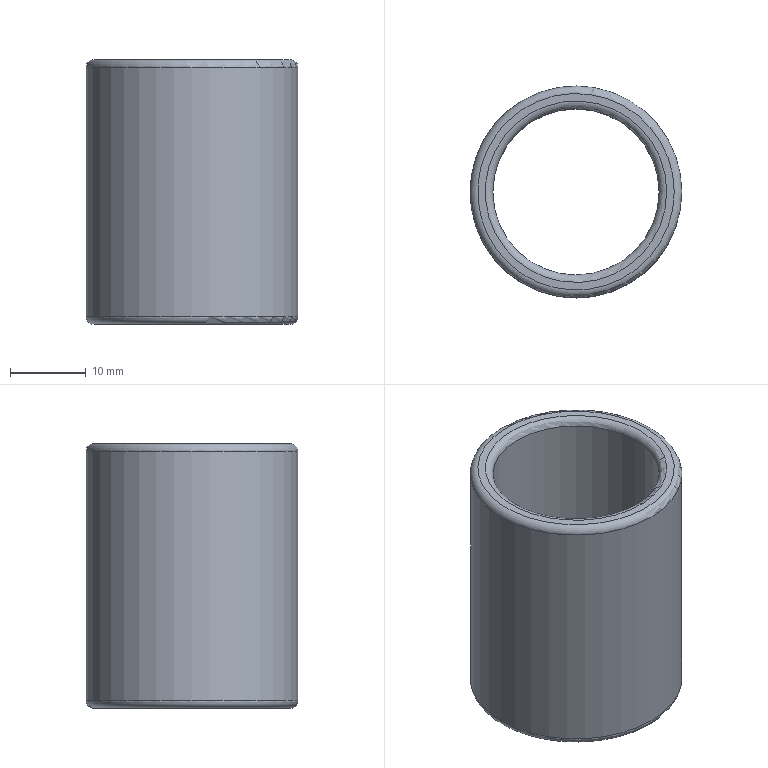Part | STEP file | 1 solid | 8 faces | box 28 x 28 x 35 mm | volume 8179 mm3 | torus 4 | plane 2 | cylinder 2 | commonest cylinder face diameters 22 x1 28 x1
STEP:
#1=CARTESIAN_POINT('',(0.,0.,0.));
#2=DIRECTION('',(0.,0.,1.));
#3=DIRECTION('',(1.,0.,0.));
#4=AXIS2_PLACEMENT_3D('',#1,#2,#3);
#5=CARTESIAN_POINT('',(1547.247,368.48,38.619));
#6=VERTEX_POINT('',#5);
#7=CARTESIAN_POINT('',(1534.247,368.48,38.619));
#8=DIRECTION('',(0.,0.,1.));
#9=DIRECTION('',(1.,0.,0.));
#10=AXIS2_PLACEMENT_3D('',#7,#8,#9);
#11=CIRCLE('',#10,13.);
#12=CARTESIAN_POINT('',(1534.247,368.48,38.619));
#13=DIRECTION('',(0.,0.,1.));
#14=DIRECTION('',(1.,0.,0.));
#15=AXIS2_PLACEMENT_3D('',#12,#13,#14);
#16=PLANE('',#15);
#17=CARTESIAN_POINT('',(0.,0.));
#18=DIRECTION('',(1.,0.));
#19=AXIS2_PLACEMENT_2D('',#17,#18);
#20=CIRCLE('',#19,13.);
#21=(GEOMETRIC_REPRESENTATION_CONTEXT(2)PARAMETRIC_REPRESENTATION_CONTEXT()REPRESENTATION_CONTEXT('',''));
#22=DEFINITIONAL_REPRESENTATION('',(#20),#21);
#23=PCURVE('',#16,#22);
#24=CARTESIAN_POINT('',(1534.247,368.48,37.619));
#25=DIRECTION('',(0.,0.,1.));
#26=DIRECTION('',(-1.,0.,0.));
#27=AXIS2_PLACEMENT_3D('',#24,#25,#26);
#28=TOROIDAL_SURFACE('',#27,13.,1.);
#29=CARTESIAN_POINT('',(3.142,7.854));
#30=DIRECTION('',(1.,0.));
#31=VECTOR('',#30,1.);
#32=LINE('',#29,#31);
#33=(GEOMETRIC_REPRESENTATION_CONTEXT(2)PARAMETRIC_REPRESENTATION_CONTEXT()REPRESENTATION_CONTEXT('',''));
#34=DEFINITIONAL_REPRESENTATION('',(#32),#33);
#35=PCURVE('',#28,#34);
#36=SURFACE_CURVE('',#11,(#23,#35),.PCURVE_S1.);
#37=EDGE_CURVE('',#6,#6,#36,.T.);
#38=ORIENTED_EDGE('',*,*,#37,.T.);
#39=EDGE_LOOP('',(#38));
#40=FACE_BOUND('',#39,.T.);
#41=CARTESIAN_POINT('',(1546.247,368.48,38.619));
#42=VERTEX_POINT('',#41);
#43=CARTESIAN_POINT('',(1534.247,368.48,38.619));
#44=DIRECTION('',(0.,0.,-1.));
#45=DIRECTION('',(1.,0.,0.));
#46=AXIS2_PLACEMENT_3D('',#43,#44,#45);
#47=CIRCLE('',#46,12.);
#48=CARTESIAN_POINT('',(12.,0.));
#49=CARTESIAN_POINT('',(12.,-20.785));
#50=CARTESIAN_POINT('',(-6.,-10.392));
#51=CARTESIAN_POINT('',(-24.,0.));
#52=CARTESIAN_POINT('',(-6.,10.392));
#53=CARTESIAN_POINT('',(12.,20.785));
#54=CARTESIAN_POINT('',(12.,0.));
#55=(BOUNDED_CURVE()B_SPLINE_CURVE(2,(#48,#49,#50,#51,#52,#53,#54),.UNSPECIFIED.,.T.,.F.)B_SPLINE_CURVE_WITH_KNOTS((1,2,2,2,2,1),(-2.094,0.,2.094,4.189,6.283,8.378),.UNSPECIFIED.)CURVE()GEOMETRIC_REPRESENTATION_ITEM()RATIONAL_B_SPLINE_CURVE((1.,0.5,1.,0.5,1.,0.5,1.))REPRESENTATION_ITEM(''));
#56=(GEOMETRIC_REPRESENTATION_CONTEXT(2)PARAMETRIC_REPRESENTATION_CONTEXT()REPRESENTATION_CONTEXT('',''));
#57=DEFINITIONAL_REPRESENTATION('',(#55),#56);
#58=PCURVE('',#16,#57);
#59=CARTESIAN_POINT('',(1534.247,368.48,37.619));
#60=DIRECTION('',(0.,0.,1.));
#61=DIRECTION('',(-1.,0.,0.));
#62=AXIS2_PLACEMENT_3D('',#59,#60,#61);
#63=TOROIDAL_SURFACE('',#62,12.,1.);
#64=CARTESIAN_POINT('',(9.425,7.854));
#65=DIRECTION('',(-1.,0.));
#66=VECTOR('',#65,1.);
#67=LINE('',#64,#66);
#68=(GEOMETRIC_REPRESENTATION_CONTEXT(2)PARAMETRIC_REPRESENTATION_CONTEXT()REPRESENTATION_CONTEXT('',''));
#69=DEFINITIONAL_REPRESENTATION('',(#67),#68);
#70=PCURVE('',#63,#69);
#71=SURFACE_CURVE('',#47,(#58,#70),.PCURVE_S1.);
#72=EDGE_CURVE('',#42,#42,#71,.T.);
#73=ORIENTED_EDGE('',*,*,#72,.T.);
#74=EDGE_LOOP('',(#73));
#75=FACE_BOUND('',#74,.T.);
#76=ADVANCED_FACE('',(#40,#75),#16,.T.);
#77=CARTESIAN_POINT('',(1548.247,368.48,37.619));
#78=VERTEX_POINT('',#77);
#79=CARTESIAN_POINT('',(1534.247,368.48,37.619));
#80=DIRECTION('',(0.,0.,-1.));
#81=DIRECTION('',(1.,0.,0.));
#82=AXIS2_PLACEMENT_3D('',#79,#80,#81);
#83=CIRCLE('',#82,14.);
#84=CARTESIAN_POINT('',(1534.247,368.48,33.619));
#85=DIRECTION('',(0.,0.,-1.));
#86=DIRECTION('',(-1.,0.,0.));
#87=AXIS2_PLACEMENT_3D('',#84,#85,#86);
#88=CYLINDRICAL_SURFACE('',#87,14.);
#89=CARTESIAN_POINT('',(3.142,-4.));
#90=DIRECTION('',(1.,0.));
#91=VECTOR('',#90,1.);
#92=LINE('',#89,#91);
#93=(GEOMETRIC_REPRESENTATION_CONTEXT(2)PARAMETRIC_REPRESENTATION_CONTEXT()REPRESENTATION_CONTEXT('',''));
#94=DEFINITIONAL_REPRESENTATION('',(#92),#93);
#95=PCURVE('',#88,#94);
#96=CARTESIAN_POINT('',(9.425,6.283));
#97=DIRECTION('',(-1.,0.));
#98=VECTOR('',#97,1.);
#99=LINE('',#96,#98);
#100=(GEOMETRIC_REPRESENTATION_CONTEXT(2)PARAMETRIC_REPRESENTATION_CONTEXT()REPRESENTATION_CONTEXT('',''));
#101=DEFINITIONAL_REPRESENTATION('',(#99),#100);
#102=PCURVE('',#28,#101);
#103=SURFACE_CURVE('',#83,(#95,#102),.PCURVE_S1.);
#104=EDGE_CURVE('',#78,#78,#103,.T.);
#105=ORIENTED_EDGE('',*,*,#104,.T.);
#106=CARTESIAN_POINT('',(1548.247,368.48,4.619));
#107=VERTEX_POINT('',#106);
#108=CARTESIAN_POINT('',(1548.247,368.48,37.619));
#109=CARTESIAN_POINT('',(1548.247,368.48,4.619));
#110=B_SPLINE_CURVE_WITH_KNOTS('',1,(#108,#109),.UNSPECIFIED.,.F.,.F.,(2,2),(-4.,29.),.PIECEWISE_BEZIER_KNOTS.);
#111=CARTESIAN_POINT('',(9.425,0.));
#112=DIRECTION('',(0.,1.));
#113=VECTOR('',#112,1.);
#114=LINE('',#111,#113);
#115=(GEOMETRIC_REPRESENTATION_CONTEXT(2)PARAMETRIC_REPRESENTATION_CONTEXT()REPRESENTATION_CONTEXT('',''));
#116=DEFINITIONAL_REPRESENTATION('',(#114),#115);
#117=PCURVE('',#88,#116);
#118=CARTESIAN_POINT('',(3.142,0.));
#119=DIRECTION('',(0.,1.));
#120=VECTOR('',#119,1.);
#121=LINE('',#118,#120);
#122=(GEOMETRIC_REPRESENTATION_CONTEXT(2)PARAMETRIC_REPRESENTATION_CONTEXT()REPRESENTATION_CONTEXT('',''));
#123=DEFINITIONAL_REPRESENTATION('',(#121),#122);
#124=PCURVE('',#88,#123);
#125=SEAM_CURVE('',#110,(#117,#124),.PCURVE_S1.);
#126=EDGE_CURVE('',#78,#107,#125,.T.);
#127=ORIENTED_EDGE('',*,*,#126,.T.);
#128=CARTESIAN_POINT('',(1534.247,368.48,4.619));
#129=DIRECTION('',(0.,0.,1.));
#130=DIRECTION('',(1.,0.,0.));
#131=AXIS2_PLACEMENT_3D('',#128,#129,#130);
#132=CIRCLE('',#131,14.);
#133=CARTESIAN_POINT('',(9.425,29.));
#134=DIRECTION('',(-1.,0.));
#135=VECTOR('',#134,1.);
#136=LINE('',#133,#135);
#137=(GEOMETRIC_REPRESENTATION_CONTEXT(2)PARAMETRIC_REPRESENTATION_CONTEXT()REPRESENTATION_CONTEXT('',''));
#138=DEFINITIONAL_REPRESENTATION('',(#136),#137);
#139=PCURVE('',#88,#138);
#140=CARTESIAN_POINT('',(1534.247,368.48,4.619));
#141=DIRECTION('',(0.,0.,1.));
#142=DIRECTION('',(-1.,0.,0.));
#143=AXIS2_PLACEMENT_3D('',#140,#141,#142);
#144=TOROIDAL_SURFACE('',#143,13.,1.);
#145=CARTESIAN_POINT('',(3.142,6.283));
#146=DIRECTION('',(1.,0.));
#147=VECTOR('',#146,1.);
#148=LINE('',#145,#147);
#149=(GEOMETRIC_REPRESENTATION_CONTEXT(2)PARAMETRIC_REPRESENTATION_CONTEXT()REPRESENTATION_CONTEXT('',''));
#150=DEFINITIONAL_REPRESENTATION('',(#148),#149);
#151=PCURVE('',#144,#150);
#152=SURFACE_CURVE('',#132,(#139,#151),.PCURVE_S1.);
#153=EDGE_CURVE('',#107,#107,#152,.T.);
#154=ORIENTED_EDGE('',*,*,#153,.T.);
#155=ORIENTED_EDGE('',*,*,#126,.F.);
#156=EDGE_LOOP('',(#105,#127,#154,#155));
#157=FACE_BOUND('',#156,.T.);
#158=ADVANCED_FACE('',(#157),#88,.T.);
#159=CARTESIAN_POINT('',(1546.247,368.48,3.619));
#160=VERTEX_POINT('',#159);
#161=CARTESIAN_POINT('',(1534.247,368.48,3.619));
#162=DIRECTION('',(0.,0.,1.));
#163=DIRECTION('',(1.,0.,0.));
#164=AXIS2_PLACEMENT_3D('',#161,#162,#163);
#165=CIRCLE('',#164,12.);
#166=CARTESIAN_POINT('',(1534.247,368.48,3.619));
#167=DIRECTION('',(0.,0.,1.));
#168=DIRECTION('',(1.,0.,0.));
#169=AXIS2_PLACEMENT_3D('',#166,#167,#168);
#170=PLANE('',#169);
#171=CARTESIAN_POINT('',(0.,0.));
#172=DIRECTION('',(1.,0.));
#173=AXIS2_PLACEMENT_2D('',#171,#172);
#174=CIRCLE('',#173,12.);
#175=(GEOMETRIC_REPRESENTATION_CONTEXT(2)PARAMETRIC_REPRESENTATION_CONTEXT()REPRESENTATION_CONTEXT('',''));
#176=DEFINITIONAL_REPRESENTATION('',(#174),#175);
#177=PCURVE('',#170,#176);
#178=CARTESIAN_POINT('',(1534.247,368.48,4.619));
#179=DIRECTION('',(0.,0.,1.));
#180=DIRECTION('',(-1.,0.,0.));
#181=AXIS2_PLACEMENT_3D('',#178,#179,#180);
#182=TOROIDAL_SURFACE('',#181,12.,1.);
#183=CARTESIAN_POINT('',(3.142,4.712));
#184=DIRECTION('',(1.,0.));
#185=VECTOR('',#184,1.);
#186=LINE('',#183,#185);
#187=(GEOMETRIC_REPRESENTATION_CONTEXT(2)PARAMETRIC_REPRESENTATION_CONTEXT()REPRESENTATION_CONTEXT('',''));
#188=DEFINITIONAL_REPRESENTATION('',(#186),#187);
#189=PCURVE('',#182,#188);
#190=SURFACE_CURVE('',#165,(#177,#189),.PCURVE_S1.);
#191=EDGE_CURVE('',#160,#160,#190,.T.);
#192=ORIENTED_EDGE('',*,*,#191,.T.);
#193=EDGE_LOOP('',(#192));
#194=FACE_BOUND('',#193,.T.);
#195=CARTESIAN_POINT('',(1547.247,368.48,3.619));
#196=VERTEX_POINT('',#195);
#197=CARTESIAN_POINT('',(1534.247,368.48,3.619));
#198=DIRECTION('',(0.,0.,-1.));
#199=DIRECTION('',(1.,0.,0.));
#200=AXIS2_PLACEMENT_3D('',#197,#198,#199);
#201=CIRCLE('',#200,13.);
#202=CARTESIAN_POINT('',(13.,0.));
#203=CARTESIAN_POINT('',(13.,-22.517));
#204=CARTESIAN_POINT('',(-6.5,-11.258));
#205=CARTESIAN_POINT('',(-26.,0.));
#206=CARTESIAN_POINT('',(-6.5,11.258));
#207=CARTESIAN_POINT('',(13.,22.517));
#208=CARTESIAN_POINT('',(13.,0.));
#209=(BOUNDED_CURVE()B_SPLINE_CURVE(2,(#202,#203,#204,#205,#206,#207,#208),.UNSPECIFIED.,.T.,.F.)B_SPLINE_CURVE_WITH_KNOTS((1,2,2,2,2,1),(-2.094,0.,2.094,4.189,6.283,8.378),.UNSPECIFIED.)CURVE()GEOMETRIC_REPRESENTATION_ITEM()RATIONAL_B_SPLINE_CURVE((1.,0.5,1.,0.5,1.,0.5,1.))REPRESENTATION_ITEM(''));
#210=(GEOMETRIC_REPRESENTATION_CONTEXT(2)PARAMETRIC_REPRESENTATION_CONTEXT()REPRESENTATION_CONTEXT('',''));
#211=DEFINITIONAL_REPRESENTATION('',(#209),#210);
#212=PCURVE('',#170,#211);
#213=CARTESIAN_POINT('',(9.425,4.712));
#214=DIRECTION('',(-1.,0.));
#215=VECTOR('',#214,1.);
#216=LINE('',#213,#215);
#217=(GEOMETRIC_REPRESENTATION_CONTEXT(2)PARAMETRIC_REPRESENTATION_CONTEXT()REPRESENTATION_CONTEXT('',''));
#218=DEFINITIONAL_REPRESENTATION('',(#216),#217);
#219=PCURVE('',#144,#218);
#220=SURFACE_CURVE('',#201,(#212,#219),.PCURVE_S1.);
#221=EDGE_CURVE('',#196,#196,#220,.T.);
#222=ORIENTED_EDGE('',*,*,#221,.T.);
#223=EDGE_LOOP('',(#222));
#224=FACE_BOUND('',#223,.T.);
#225=ADVANCED_FACE('',(#194,#224),#170,.F.);
#226=CARTESIAN_POINT('',(1545.247,368.48,37.619));
#227=VERTEX_POINT('',#226);
#228=CARTESIAN_POINT('',(1534.247,368.48,37.619));
#229=DIRECTION('',(0.,0.,1.));
#230=DIRECTION('',(1.,0.,0.));
#231=AXIS2_PLACEMENT_3D('',#228,#229,#230);
#232=CIRCLE('',#231,11.);
#233=CARTESIAN_POINT('',(1534.247,368.48,33.619));
#234=DIRECTION('',(0.,0.,-1.));
#235=DIRECTION('',(-1.,0.,0.));
#236=AXIS2_PLACEMENT_3D('',#233,#234,#235);
#237=CYLINDRICAL_SURFACE('',#236,11.);
#238=CARTESIAN_POINT('',(9.425,-4.));
#239=DIRECTION('',(-1.,0.));
#240=VECTOR('',#239,1.);
#241=LINE('',#238,#240);
#242=(GEOMETRIC_REPRESENTATION_CONTEXT(2)PARAMETRIC_REPRESENTATION_CONTEXT()REPRESENTATION_CONTEXT('',''));
#243=DEFINITIONAL_REPRESENTATION('',(#241),#242);
#244=PCURVE('',#237,#243);
#245=CARTESIAN_POINT('',(3.142,9.425));
#246=DIRECTION('',(1.,0.));
#247=VECTOR('',#246,1.);
#248=LINE('',#245,#247);
#249=(GEOMETRIC_REPRESENTATION_CONTEXT(2)PARAMETRIC_REPRESENTATION_CONTEXT()REPRESENTATION_CONTEXT('',''));
#250=DEFINITIONAL_REPRESENTATION('',(#248),#249);
#251=PCURVE('',#63,#250);
#252=SURFACE_CURVE('',#232,(#244,#251),.PCURVE_S1.);
#253=EDGE_CURVE('',#227,#227,#252,.T.);
#254=ORIENTED_EDGE('',*,*,#253,.F.);
#255=CARTESIAN_POINT('',(1545.247,368.48,4.619));
#256=VERTEX_POINT('',#255);
#257=CARTESIAN_POINT('',(1545.247,368.48,37.619));
#258=CARTESIAN_POINT('',(1545.247,368.48,4.619));
#259=B_SPLINE_CURVE_WITH_KNOTS('',1,(#257,#258),.UNSPECIFIED.,.F.,.F.,(2,2),(-4.,29.),.PIECEWISE_BEZIER_KNOTS.);
#260=CARTESIAN_POINT('',(9.425,0.));
#261=DIRECTION('',(0.,1.));
#262=VECTOR('',#261,1.);
#263=LINE('',#260,#262);
#264=(GEOMETRIC_REPRESENTATION_CONTEXT(2)PARAMETRIC_REPRESENTATION_CONTEXT()REPRESENTATION_CONTEXT('',''));
#265=DEFINITIONAL_REPRESENTATION('',(#263),#264);
#266=PCURVE('',#237,#265);
#267=CARTESIAN_POINT('',(3.142,0.));
#268=DIRECTION('',(0.,1.));
#269=VECTOR('',#268,1.);
#270=LINE('',#267,#269);
#271=(GEOMETRIC_REPRESENTATION_CONTEXT(2)PARAMETRIC_REPRESENTATION_CONTEXT()REPRESENTATION_CONTEXT('',''));
#272=DEFINITIONAL_REPRESENTATION('',(#270),#271);
#273=PCURVE('',#237,#272);
#274=SEAM_CURVE('',#259,(#266,#273),.PCURVE_S1.);
#275=EDGE_CURVE('',#227,#256,#274,.T.);
#276=ORIENTED_EDGE('',*,*,#275,.T.);
#277=CARTESIAN_POINT('',(1534.247,368.48,4.619));
#278=DIRECTION('',(0.,0.,-1.));
#279=DIRECTION('',(1.,0.,0.));
#280=AXIS2_PLACEMENT_3D('',#277,#278,#279);
#281=CIRCLE('',#280,11.);
#282=CARTESIAN_POINT('',(3.142,29.));
#283=DIRECTION('',(1.,0.));
#284=VECTOR('',#283,1.);
#285=LINE('',#282,#284);
#286=(GEOMETRIC_REPRESENTATION_CONTEXT(2)PARAMETRIC_REPRESENTATION_CONTEXT()REPRESENTATION_CONTEXT('',''));
#287=DEFINITIONAL_REPRESENTATION('',(#285),#286);
#288=PCURVE('',#237,#287);
#289=CARTESIAN_POINT('',(9.425,3.142));
#290=DIRECTION('',(-1.,0.));
#291=VECTOR('',#290,1.);
#292=LINE('',#289,#291);
#293=(GEOMETRIC_REPRESENTATION_CONTEXT(2)PARAMETRIC_REPRESENTATION_CONTEXT()REPRESENTATION_CONTEXT('',''));
#294=DEFINITIONAL_REPRESENTATION('',(#292),#293);
#295=PCURVE('',#182,#294);
#296=SURFACE_CURVE('',#281,(#288,#295),.PCURVE_S1.);
#297=EDGE_CURVE('',#256,#256,#296,.T.);
#298=ORIENTED_EDGE('',*,*,#297,.F.);
#299=ORIENTED_EDGE('',*,*,#275,.F.);
#300=EDGE_LOOP('',(#254,#276,#298,#299));
#301=FACE_BOUND('',#300,.F.);
#302=ADVANCED_FACE('',(#301),#237,.F.);
#303=ORIENTED_EDGE('',*,*,#104,.F.);
#304=CARTESIAN_POINT('',(1548.247,368.48,37.619));
#305=CARTESIAN_POINT('',(1548.247,368.48,37.886));
#306=CARTESIAN_POINT('',(1548.162,368.48,38.147));
#307=CARTESIAN_POINT('',(1547.999,368.48,38.371));
#308=CARTESIAN_POINT('',(1547.775,368.48,38.534));
#309=CARTESIAN_POINT('',(1547.515,368.48,38.619));
#310=CARTESIAN_POINT('',(1547.247,368.48,38.619));
#311=(BOUNDED_CURVE()B_SPLINE_CURVE(6,(#304,#305,#306,#307,#308,#309,#310),.UNSPECIFIED.,.F.,.F.)B_SPLINE_CURVE_WITH_KNOTS((7,7),(0.,1.571),.PIECEWISE_BEZIER_KNOTS.)CURVE()GEOMETRIC_REPRESENTATION_ITEM()RATIONAL_B_SPLINE_CURVE((1.031,1.01,0.9979,0.994,0.9979,1.01,1.031))REPRESENTATION_ITEM(''));
#312=CARTESIAN_POINT('',(9.425,6.283));
#313=DIRECTION('',(0.,1.));
#314=VECTOR('',#313,1.);
#315=LINE('',#312,#314);
#316=(GEOMETRIC_REPRESENTATION_CONTEXT(2)PARAMETRIC_REPRESENTATION_CONTEXT()REPRESENTATION_CONTEXT('',''));
#317=DEFINITIONAL_REPRESENTATION('',(#315),#316);
#318=PCURVE('',#28,#317);
#319=CARTESIAN_POINT('',(3.142,6.283));
#320=DIRECTION('',(0.,1.));
#321=VECTOR('',#320,1.);
#322=LINE('',#319,#321);
#323=(GEOMETRIC_REPRESENTATION_CONTEXT(2)PARAMETRIC_REPRESENTATION_CONTEXT()REPRESENTATION_CONTEXT('',''));
#324=DEFINITIONAL_REPRESENTATION('',(#322),#323);
#325=PCURVE('',#28,#324);
#326=SEAM_CURVE('',#311,(#318,#325),.PCURVE_S1.);
#327=EDGE_CURVE('',#78,#6,#326,.T.);
#328=ORIENTED_EDGE('',*,*,#327,.T.);
#329=ORIENTED_EDGE('',*,*,#37,.F.);
#330=ORIENTED_EDGE('',*,*,#327,.F.);
#331=EDGE_LOOP('',(#303,#328,#329,#330));
#332=FACE_BOUND('',#331,.T.);
#333=ADVANCED_FACE('',(#332),#28,.T.);
#334=ORIENTED_EDGE('',*,*,#253,.F.);
#335=CARTESIAN_POINT('',(1546.247,368.48,38.619));
#336=CARTESIAN_POINT('',(1545.98,368.48,38.619));
#337=CARTESIAN_POINT('',(1545.719,368.48,38.534));
#338=CARTESIAN_POINT('',(1545.495,368.48,38.371));
#339=CARTESIAN_POINT('',(1545.332,368.48,38.147));
#340=CARTESIAN_POINT('',(1545.247,368.48,37.886));
#341=CARTESIAN_POINT('',(1545.247,368.48,37.619));
#342=(BOUNDED_CURVE()B_SPLINE_CURVE(6,(#335,#336,#337,#338,#339,#340,#341),.UNSPECIFIED.,.F.,.F.)B_SPLINE_CURVE_WITH_KNOTS((7,7),(1.571,3.142),.PIECEWISE_BEZIER_KNOTS.)CURVE()GEOMETRIC_REPRESENTATION_ITEM()RATIONAL_B_SPLINE_CURVE((1.031,1.01,0.9979,0.994,0.9979,1.01,1.031))REPRESENTATION_ITEM(''));
#343=CARTESIAN_POINT('',(3.142,6.283));
#344=DIRECTION('',(0.,1.));
#345=VECTOR('',#344,1.);
#346=LINE('',#343,#345);
#347=(GEOMETRIC_REPRESENTATION_CONTEXT(2)PARAMETRIC_REPRESENTATION_CONTEXT()REPRESENTATION_CONTEXT('',''));
#348=DEFINITIONAL_REPRESENTATION('',(#346),#347);
#349=PCURVE('',#63,#348);
#350=CARTESIAN_POINT('',(9.425,6.283));
#351=DIRECTION('',(0.,1.));
#352=VECTOR('',#351,1.);
#353=LINE('',#350,#352);
#354=(GEOMETRIC_REPRESENTATION_CONTEXT(2)PARAMETRIC_REPRESENTATION_CONTEXT()REPRESENTATION_CONTEXT('',''));
#355=DEFINITIONAL_REPRESENTATION('',(#353),#354);
#356=PCURVE('',#63,#355);
#357=SEAM_CURVE('',#342,(#349,#356),.PCURVE_S1.);
#358=EDGE_CURVE('',#42,#227,#357,.T.);
#359=ORIENTED_EDGE('',*,*,#358,.F.);
#360=ORIENTED_EDGE('',*,*,#72,.F.);
#361=ORIENTED_EDGE('',*,*,#358,.T.);
#362=EDGE_LOOP('',(#334,#359,#360,#361));
#363=FACE_BOUND('',#362,.T.);
#364=ADVANCED_FACE('',(#363),#63,.T.);
#365=ORIENTED_EDGE('',*,*,#297,.F.);
#366=CARTESIAN_POINT('',(1545.247,368.48,4.619));
#367=CARTESIAN_POINT('',(1545.247,368.48,4.352));
#368=CARTESIAN_POINT('',(1545.332,368.48,4.091));
#369=CARTESIAN_POINT('',(1545.495,368.48,3.867));
#370=CARTESIAN_POINT('',(1545.719,368.48,3.704));
#371=CARTESIAN_POINT('',(1545.98,368.48,3.619));
#372=CARTESIAN_POINT('',(1546.247,368.48,3.619));
#373=(BOUNDED_CURVE()B_SPLINE_CURVE(6,(#366,#367,#368,#369,#370,#371,#372),.UNSPECIFIED.,.F.,.F.)B_SPLINE_CURVE_WITH_KNOTS((7,7),(3.142,4.712),.PIECEWISE_BEZIER_KNOTS.)CURVE()GEOMETRIC_REPRESENTATION_ITEM()RATIONAL_B_SPLINE_CURVE((1.031,1.01,0.9979,0.994,0.9979,1.01,1.031))REPRESENTATION_ITEM(''));
#374=CARTESIAN_POINT('',(9.425,0.));
#375=DIRECTION('',(0.,1.));
#376=VECTOR('',#375,1.);
#377=LINE('',#374,#376);
#378=(GEOMETRIC_REPRESENTATION_CONTEXT(2)PARAMETRIC_REPRESENTATION_CONTEXT()REPRESENTATION_CONTEXT('',''));
#379=DEFINITIONAL_REPRESENTATION('',(#377),#378);
#380=PCURVE('',#182,#379);
#381=CARTESIAN_POINT('',(3.142,0.));
#382=DIRECTION('',(0.,1.));
#383=VECTOR('',#382,1.);
#384=LINE('',#381,#383);
#385=(GEOMETRIC_REPRESENTATION_CONTEXT(2)PARAMETRIC_REPRESENTATION_CONTEXT()REPRESENTATION_CONTEXT('',''));
#386=DEFINITIONAL_REPRESENTATION('',(#384),#385);
#387=PCURVE('',#182,#386);
#388=SEAM_CURVE('',#373,(#380,#387),.PCURVE_S1.);
#389=EDGE_CURVE('',#256,#160,#388,.T.);
#390=ORIENTED_EDGE('',*,*,#389,.T.);
#391=ORIENTED_EDGE('',*,*,#191,.F.);
#392=ORIENTED_EDGE('',*,*,#389,.F.);
#393=EDGE_LOOP('',(#365,#390,#391,#392));
#394=FACE_BOUND('',#393,.T.);
#395=ADVANCED_FACE('',(#394),#182,.T.);
#396=ORIENTED_EDGE('',*,*,#221,.F.);
#397=CARTESIAN_POINT('',(1547.247,368.48,3.619));
#398=CARTESIAN_POINT('',(1547.515,368.48,3.619));
#399=CARTESIAN_POINT('',(1547.775,368.48,3.704));
#400=CARTESIAN_POINT('',(1547.999,368.48,3.867));
#401=CARTESIAN_POINT('',(1548.162,368.48,4.091));
#402=CARTESIAN_POINT('',(1548.247,368.48,4.352));
#403=CARTESIAN_POINT('',(1548.247,368.48,4.619));
#404=(BOUNDED_CURVE()B_SPLINE_CURVE(6,(#397,#398,#399,#400,#401,#402,#403),.UNSPECIFIED.,.F.,.F.)B_SPLINE_CURVE_WITH_KNOTS((7,7),(4.712,6.283),.PIECEWISE_BEZIER_KNOTS.)CURVE()GEOMETRIC_REPRESENTATION_ITEM()RATIONAL_B_SPLINE_CURVE((1.031,1.01,0.9979,0.994,0.9979,1.01,1.031))REPRESENTATION_ITEM(''));
#405=CARTESIAN_POINT('',(9.425,0.));
#406=DIRECTION('',(0.,1.));
#407=VECTOR('',#406,1.);
#408=LINE('',#405,#407);
#409=(GEOMETRIC_REPRESENTATION_CONTEXT(2)PARAMETRIC_REPRESENTATION_CONTEXT()REPRESENTATION_CONTEXT('',''));
#410=DEFINITIONAL_REPRESENTATION('',(#408),#409);
#411=PCURVE('',#144,#410);
#412=CARTESIAN_POINT('',(3.142,0.));
#413=DIRECTION('',(0.,1.));
#414=VECTOR('',#413,1.);
#415=LINE('',#412,#414);
#416=(GEOMETRIC_REPRESENTATION_CONTEXT(2)PARAMETRIC_REPRESENTATION_CONTEXT()REPRESENTATION_CONTEXT('',''));
#417=DEFINITIONAL_REPRESENTATION('',(#415),#416);
#418=PCURVE('',#144,#417);
#419=SEAM_CURVE('',#404,(#411,#418),.PCURVE_S1.);
#420=EDGE_CURVE('',#196,#107,#419,.T.);
#421=ORIENTED_EDGE('',*,*,#420,.T.);
#422=ORIENTED_EDGE('',*,*,#153,.F.);
#423=ORIENTED_EDGE('',*,*,#420,.F.);
#424=EDGE_LOOP('',(#396,#421,#422,#423));
#425=FACE_BOUND('',#424,.T.);
#426=ADVANCED_FACE('',(#425),#144,.T.);
#427=CLOSED_SHELL('',(#76,#158,#225,#302,#333,#364,#395,#426));
#428=MANIFOLD_SOLID_BREP('',#427);
#429=(LENGTH_UNIT()NAMED_UNIT(*)SI_UNIT(.MILLI.,.METRE.));
#430=UNCERTAINTY_MEASURE_WITH_UNIT(LENGTH_MEASURE(0.00001),#429,'','');
#431=(NAMED_UNIT(*)PLANE_ANGLE_UNIT()SI_UNIT($,.RADIAN.));
#432=(NAMED_UNIT(*)SI_UNIT($,.STERADIAN.)SOLID_ANGLE_UNIT());
#433=(GEOMETRIC_REPRESENTATION_CONTEXT(3)GLOBAL_UNCERTAINTY_ASSIGNED_CONTEXT((#430))GLOBAL_UNIT_ASSIGNED_CONTEXT((#429,#431,#432))REPRESENTATION_CONTEXT('',''));
#434=ADVANCED_BREP_SHAPE_REPRESENTATION('',(#4,#428),#433);